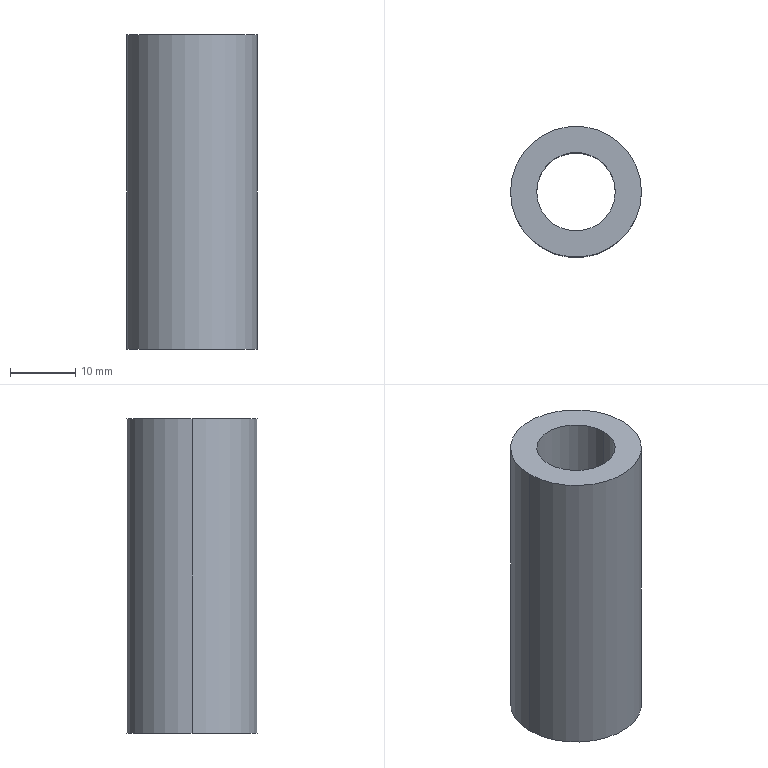Part | SolidWorks | features Extrusion 1 | 1 solid | 6 faces | box 20 x 20 x 48 mm | volume 9651 mm3 | cylinder 4 | plane 2 | commonest cylinder face diameters 12 x2 20 x2
STEP:
#1=CARTESIAN_POINT('',(-6.,0.,48.));
#2=VERTEX_POINT('',#1);
#3=CARTESIAN_POINT('',(6.,0.,48.));
#4=VERTEX_POINT('',#3);
#5=CARTESIAN_POINT('',(0.,0.,48.));
#6=DIRECTION('',(0.,0.,1.));
#7=DIRECTION('',(1.,0.,0.));
#8=AXIS2_PLACEMENT_3D('',#5,#6,#7);
#9=CIRCLE('',#8,6.);
#10=EDGE_CURVE('',#2,#4,#9,.T.);
#11=ORIENTED_EDGE('',*,*,#10,.T.);
#12=CARTESIAN_POINT('',(6.,0.,0.));
#13=VERTEX_POINT('',#12);
#14=CARTESIAN_POINT('',(6.,0.,48.));
#15=DIRECTION('',(0.,0.,-1.));
#16=VECTOR('',#15,1000.);
#17=LINE('',#14,#16);
#18=EDGE_CURVE('',#4,#13,#17,.T.);
#19=ORIENTED_EDGE('',*,*,#18,.T.);
#20=CARTESIAN_POINT('',(-6.,0.,0.));
#21=VERTEX_POINT('',#20);
#22=CARTESIAN_POINT('',(0.,0.,0.));
#23=DIRECTION('',(0.,0.,1.));
#24=DIRECTION('',(1.,0.,0.));
#25=AXIS2_PLACEMENT_3D('',#22,#23,#24);
#26=CIRCLE('',#25,6.);
#27=EDGE_CURVE('',#21,#13,#26,.T.);
#28=ORIENTED_EDGE('',*,*,#27,.F.);
#29=CARTESIAN_POINT('',(-6.,0.,48.));
#30=DIRECTION('',(0.,0.,-1.));
#31=VECTOR('',#30,1000.);
#32=LINE('',#29,#31);
#33=EDGE_CURVE('',#2,#21,#32,.T.);
#34=ORIENTED_EDGE('',*,*,#33,.F.);
#35=EDGE_LOOP('',(#11,#19,#28,#34));
#36=FACE_OUTER_BOUND('',#35,.T.);
#37=CARTESIAN_POINT('',(0.,0.,48.));
#38=DIRECTION('',(0.,0.,-1.));
#39=DIRECTION('',(-1.,0.,0.));
#40=AXIS2_PLACEMENT_3D('',#37,#38,#39);
#41=CYLINDRICAL_SURFACE('',#40,6.);
#42=ADVANCED_FACE('',(#36),#41,.F.);
#43=CARTESIAN_POINT('',(10.,0.,48.));
#44=VERTEX_POINT('',#43);
#45=CARTESIAN_POINT('',(-10.,0.,48.));
#46=VERTEX_POINT('',#45);
#47=CARTESIAN_POINT('',(0.,0.,48.));
#48=DIRECTION('',(0.,0.,1.));
#49=DIRECTION('',(1.,0.,0.));
#50=AXIS2_PLACEMENT_3D('',#47,#48,#49);
#51=CIRCLE('',#50,10.);
#52=EDGE_CURVE('',#44,#46,#51,.T.);
#53=ORIENTED_EDGE('',*,*,#52,.F.);
#54=CARTESIAN_POINT('',(10.,0.,0.));
#55=VERTEX_POINT('',#54);
#56=CARTESIAN_POINT('',(10.,0.,48.));
#57=DIRECTION('',(0.,0.,-1.));
#58=VECTOR('',#57,1000.);
#59=LINE('',#56,#58);
#60=EDGE_CURVE('',#44,#55,#59,.T.);
#61=ORIENTED_EDGE('',*,*,#60,.T.);
#62=CARTESIAN_POINT('',(-10.,0.,0.));
#63=VERTEX_POINT('',#62);
#64=CARTESIAN_POINT('',(0.,0.,0.));
#65=DIRECTION('',(0.,0.,1.));
#66=DIRECTION('',(1.,0.,0.));
#67=AXIS2_PLACEMENT_3D('',#64,#65,#66);
#68=CIRCLE('',#67,10.);
#69=EDGE_CURVE('',#55,#63,#68,.T.);
#70=ORIENTED_EDGE('',*,*,#69,.T.);
#71=CARTESIAN_POINT('',(-10.,0.,48.));
#72=DIRECTION('',(0.,0.,-1.));
#73=VECTOR('',#72,1000.);
#74=LINE('',#71,#73);
#75=EDGE_CURVE('',#46,#63,#74,.T.);
#76=ORIENTED_EDGE('',*,*,#75,.F.);
#77=EDGE_LOOP('',(#53,#61,#70,#76));
#78=FACE_OUTER_BOUND('',#77,.T.);
#79=CARTESIAN_POINT('',(0.,0.,48.));
#80=DIRECTION('',(0.,0.,-1.));
#81=DIRECTION('',(-1.,0.,0.));
#82=AXIS2_PLACEMENT_3D('',#79,#80,#81);
#83=CYLINDRICAL_SURFACE('',#82,10.);
#84=ADVANCED_FACE('',(#78),#83,.T.);
#85=CARTESIAN_POINT('',(0.,0.,48.));
#86=DIRECTION('',(0.,0.,1.));
#87=DIRECTION('',(1.,0.,0.));
#88=AXIS2_PLACEMENT_3D('',#85,#86,#87);
#89=CIRCLE('',#88,10.);
#90=EDGE_CURVE('',#46,#44,#89,.T.);
#91=ORIENTED_EDGE('',*,*,#90,.T.);
#92=ORIENTED_EDGE('',*,*,#52,.T.);
#93=EDGE_LOOP('',(#91,#92));
#94=FACE_OUTER_BOUND('',#93,.T.);
#95=ORIENTED_EDGE('',*,*,#10,.F.);
#96=CARTESIAN_POINT('',(0.,0.,48.));
#97=DIRECTION('',(0.,0.,1.));
#98=DIRECTION('',(1.,0.,0.));
#99=AXIS2_PLACEMENT_3D('',#96,#97,#98);
#100=CIRCLE('',#99,6.);
#101=EDGE_CURVE('',#4,#2,#100,.T.);
#102=ORIENTED_EDGE('',*,*,#101,.F.);
#103=EDGE_LOOP('',(#95,#102));
#104=FACE_BOUND('',#103,.T.);
#105=CARTESIAN_POINT('',(0.,0.,48.));
#106=DIRECTION('',(0.,0.,1.));
#107=DIRECTION('',(1.,0.,0.));
#108=AXIS2_PLACEMENT_3D('',#105,#106,#107);
#109=PLANE('',#108);
#110=ADVANCED_FACE('',(#94,#104),#109,.T.);
#111=CARTESIAN_POINT('',(0.,0.,0.));
#112=DIRECTION('',(0.,0.,1.));
#113=DIRECTION('',(1.,0.,0.));
#114=AXIS2_PLACEMENT_3D('',#111,#112,#113);
#115=CIRCLE('',#114,10.);
#116=EDGE_CURVE('',#63,#55,#115,.T.);
#117=ORIENTED_EDGE('',*,*,#116,.F.);
#118=ORIENTED_EDGE('',*,*,#69,.F.);
#119=EDGE_LOOP('',(#117,#118));
#120=FACE_OUTER_BOUND('',#119,.T.);
#121=ORIENTED_EDGE('',*,*,#27,.T.);
#122=CARTESIAN_POINT('',(0.,0.,0.));
#123=DIRECTION('',(0.,0.,1.));
#124=DIRECTION('',(1.,0.,0.));
#125=AXIS2_PLACEMENT_3D('',#122,#123,#124);
#126=CIRCLE('',#125,6.);
#127=EDGE_CURVE('',#13,#21,#126,.T.);
#128=ORIENTED_EDGE('',*,*,#127,.T.);
#129=EDGE_LOOP('',(#121,#128));
#130=FACE_BOUND('',#129,.T.);
#131=CARTESIAN_POINT('',(0.,0.,0.));
#132=DIRECTION('',(0.,0.,1.));
#133=DIRECTION('',(1.,0.,0.));
#134=AXIS2_PLACEMENT_3D('',#131,#132,#133);
#135=PLANE('',#134);
#136=ADVANCED_FACE('',(#120,#130),#135,.F.);
#137=ORIENTED_EDGE('',*,*,#60,.F.);
#138=ORIENTED_EDGE('',*,*,#90,.F.);
#139=ORIENTED_EDGE('',*,*,#75,.T.);
#140=ORIENTED_EDGE('',*,*,#116,.T.);
#141=EDGE_LOOP('',(#137,#138,#139,#140));
#142=FACE_OUTER_BOUND('',#141,.T.);
#143=CARTESIAN_POINT('',(0.,0.,48.));
#144=DIRECTION('',(0.,0.,-1.));
#145=DIRECTION('',(-1.,0.,0.));
#146=AXIS2_PLACEMENT_3D('',#143,#144,#145);
#147=CYLINDRICAL_SURFACE('',#146,10.);
#148=ADVANCED_FACE('',(#142),#147,.T.);
#149=ORIENTED_EDGE('',*,*,#18,.F.);
#150=ORIENTED_EDGE('',*,*,#101,.T.);
#151=ORIENTED_EDGE('',*,*,#33,.T.);
#152=ORIENTED_EDGE('',*,*,#127,.F.);
#153=EDGE_LOOP('',(#149,#150,#151,#152));
#154=FACE_OUTER_BOUND('',#153,.T.);
#155=CARTESIAN_POINT('',(0.,0.,48.));
#156=DIRECTION('',(0.,0.,-1.));
#157=DIRECTION('',(-1.,0.,0.));
#158=AXIS2_PLACEMENT_3D('',#155,#156,#157);
#159=CYLINDRICAL_SURFACE('',#158,6.);
#160=ADVANCED_FACE('',(#154),#159,.F.);
#161=CLOSED_SHELL('',(#42,#84,#110,#136,#148,#160));
#162=MANIFOLD_SOLID_BREP('',#161);
#163=CARTESIAN_POINT('',(0.,0.,0.));
#164=DIRECTION('',(0.,0.,1.));
#165=DIRECTION('',(1.,0.,0.));
#166=AXIS2_PLACEMENT_3D('',#163,#164,#165);
#167=(LENGTH_UNIT()NAMED_UNIT(*)SI_UNIT(.MILLI.,.METRE.));
#168=UNCERTAINTY_MEASURE_WITH_UNIT(LENGTH_MEASURE(0.00001),#167,'','');
#169=(NAMED_UNIT(*)PLANE_ANGLE_UNIT()SI_UNIT($,.RADIAN.));
#170=(NAMED_UNIT(*)SI_UNIT($,.STERADIAN.)SOLID_ANGLE_UNIT());
#171=(GEOMETRIC_REPRESENTATION_CONTEXT(3)GLOBAL_UNCERTAINTY_ASSIGNED_CONTEXT((#168))GLOBAL_UNIT_ASSIGNED_CONTEXT((#167,#169,#170))REPRESENTATION_CONTEXT('',''));
#172=ADVANCED_BREP_SHAPE_REPRESENTATION('',(#162,#166),#171);